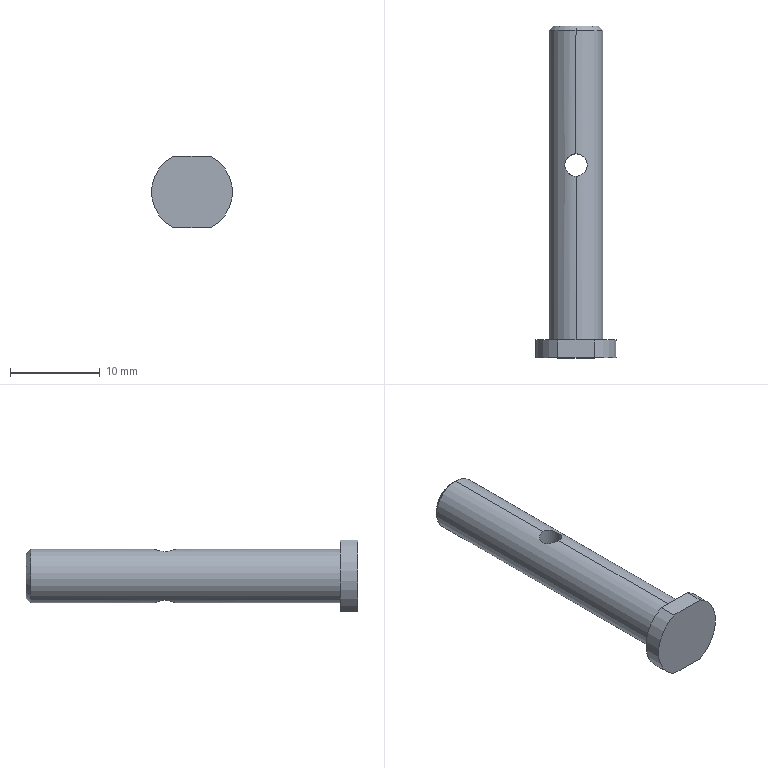Part | STEP file | 02-15 tensioning shaft | 1 solid | 13 faces | box 9 x 37 x 8 mm | volume 1080 mm3 | cylinder 6 | plane 5 | cone 2 | commonest cylinder face diameters 2.5 x2 6 x2 9 x2
STEP:
#1=CARTESIAN_POINT('',(0.,20.25,-3.));
#2=VERTEX_POINT('',#1);
#3=CARTESIAN_POINT('',(-1.25,21.5,-2.727));
#4=VERTEX_POINT('',#3);
#5=CARTESIAN_POINT('',(0.,20.25,-3.));
#6=CARTESIAN_POINT('',(-0.1646,20.25,-3.));
#7=CARTESIAN_POINT('',(-0.3304,20.283,-2.986));
#8=CARTESIAN_POINT('',(-0.6332,20.41,-2.936));
#9=CARTESIAN_POINT('',(-0.7698,20.502,-2.902));
#10=CARTESIAN_POINT('',(-0.9422,20.675,-2.849));
#11=CARTESIAN_POINT('',(-0.9933,20.737,-2.831));
#12=CARTESIAN_POINT('',(-1.083,20.871,-2.798));
#13=CARTESIAN_POINT('',(-1.122,20.944,-2.782));
#14=CARTESIAN_POINT('',(-1.185,21.094,-2.756));
#15=CARTESIAN_POINT('',(-1.209,21.172,-2.746));
#16=CARTESIAN_POINT('',(-1.242,21.334,-2.731));
#17=CARTESIAN_POINT('',(-1.25,21.418,-2.727));
#18=CARTESIAN_POINT('',(-1.25,21.5,-2.727));
#19=B_SPLINE_CURVE_WITH_KNOTS('',3,(#5,#6,#7,#8,#9,#10,#11,#12,#13,#14,#15,#16,#17,#18),.UNSPECIFIED.,.F.,.F.,(4,2,2,2,2,2,4),(0.003954,0.004448,0.004941,0.005188,0.005435,0.005682,0.005929),.UNSPECIFIED.);
#20=EDGE_CURVE('',#2,#4,#19,.T.);
#21=ORIENTED_EDGE('',*,*,#20,.T.);
#22=CARTESIAN_POINT('',(-1.25,21.5,2.727));
#23=VERTEX_POINT('',#22);
#24=CARTESIAN_POINT('',(-1.25,21.5,-6.));
#25=DIRECTION('',(0.,0.,1.));
#26=VECTOR('',#25,1000.);
#27=LINE('',#24,#26);
#28=EDGE_CURVE('',#4,#23,#27,.T.);
#29=ORIENTED_EDGE('',*,*,#28,.T.);
#30=CARTESIAN_POINT('',(0.,20.25,3.));
#31=VERTEX_POINT('',#30);
#32=CARTESIAN_POINT('',(-1.25,21.5,2.727));
#33=CARTESIAN_POINT('',(-1.25,21.335,2.727));
#34=CARTESIAN_POINT('',(-1.217,21.17,2.743));
#35=CARTESIAN_POINT('',(-1.09,20.867,2.796));
#36=CARTESIAN_POINT('',(-0.9986,20.731,2.831));
#37=CARTESIAN_POINT('',(-0.8261,20.558,2.885));
#38=CARTESIAN_POINT('',(-0.7638,20.507,2.902));
#39=CARTESIAN_POINT('',(-0.6296,20.417,2.934));
#40=CARTESIAN_POINT('',(-0.5566,20.378,2.949));
#41=CARTESIAN_POINT('',(-0.4058,20.315,2.973));
#42=CARTESIAN_POINT('',(-0.3277,20.291,2.983));
#43=CARTESIAN_POINT('',(-0.1662,20.258,2.996));
#44=CARTESIAN_POINT('',(-0.08241,20.25,3.));
#45=CARTESIAN_POINT('',(0.,20.25,3.));
#46=B_SPLINE_CURVE_WITH_KNOTS('',3,(#32,#33,#34,#35,#36,#37,#38,#39,#40,#41,#42,#43,#44,#45),.UNSPECIFIED.,.F.,.F.,(4,2,2,2,2,2,4),(0.003953,0.004447,0.004941,0.005188,0.005435,0.005682,0.005929),.UNSPECIFIED.);
#47=EDGE_CURVE('',#23,#31,#46,.T.);
#48=ORIENTED_EDGE('',*,*,#47,.T.);
#49=CARTESIAN_POINT('',(1.25,21.5,2.727));
#50=VERTEX_POINT('',#49);
#51=CARTESIAN_POINT('',(0.,20.25,3.));
#52=CARTESIAN_POINT('',(0.1648,20.25,3.));
#53=CARTESIAN_POINT('',(0.3309,20.284,2.986));
#54=CARTESIAN_POINT('',(0.6322,20.409,2.937));
#55=CARTESIAN_POINT('',(0.7695,20.502,2.902));
#56=CARTESIAN_POINT('',(0.9988,20.731,2.831));
#57=CARTESIAN_POINT('',(1.09,20.866,2.796));
#58=CARTESIAN_POINT('',(1.217,21.171,2.743));
#59=CARTESIAN_POINT('',(1.25,21.333,2.727));
#60=CARTESIAN_POINT('',(1.25,21.5,2.727));
#61=B_SPLINE_CURVE_WITH_KNOTS('',3,(#51,#52,#53,#54,#55,#56,#57,#58,#59,#60),.UNSPECIFIED.,.F.,.F.,(4,2,2,2,4),(0.005929,0.006423,0.006916,0.00741,0.007904),.UNSPECIFIED.);
#62=EDGE_CURVE('',#31,#50,#61,.T.);
#63=ORIENTED_EDGE('',*,*,#62,.T.);
#64=CARTESIAN_POINT('',(1.25,21.5,-2.727));
#65=VERTEX_POINT('',#64);
#66=CARTESIAN_POINT('',(1.25,21.5,-6.));
#67=DIRECTION('',(0.,0.,1.));
#68=VECTOR('',#67,1000.);
#69=LINE('',#66,#68);
#70=EDGE_CURVE('',#65,#50,#69,.T.);
#71=ORIENTED_EDGE('',*,*,#70,.F.);
#72=CARTESIAN_POINT('',(1.25,21.5,-2.727));
#73=CARTESIAN_POINT('',(1.25,21.417,-2.727));
#74=CARTESIAN_POINT('',(1.242,21.334,-2.731));
#75=CARTESIAN_POINT('',(1.209,21.172,-2.746));
#76=CARTESIAN_POINT('',(1.185,21.094,-2.756));
#77=CARTESIAN_POINT('',(1.09,20.866,-2.796));
#78=CARTESIAN_POINT('',(0.9976,20.73,-2.832));
#79=CARTESIAN_POINT('',(0.7691,20.501,-2.902));
#80=CARTESIAN_POINT('',(0.6313,20.409,-2.937));
#81=CARTESIAN_POINT('',(0.3309,20.284,-2.986));
#82=CARTESIAN_POINT('',(0.1647,20.25,-3.));
#83=CARTESIAN_POINT('',(0.,20.25,-3.));
#84=B_SPLINE_CURVE_WITH_KNOTS('',3,(#72,#73,#74,#75,#76,#77,#78,#79,#80,#81,#82,#83),.UNSPECIFIED.,.F.,.F.,(4,2,2,2,2,4),(0.001978,0.002225,0.002472,0.002966,0.00346,0.003954),.UNSPECIFIED.);
#85=EDGE_CURVE('',#65,#2,#84,.T.);
#86=ORIENTED_EDGE('',*,*,#85,.T.);
#87=EDGE_LOOP('',(#21,#29,#48,#63,#71,#86));
#88=FACE_OUTER_BOUND('',#87,.T.);
#89=CARTESIAN_POINT('',(0.,21.5,-6.));
#90=DIRECTION('',(0.,0.,1.));
#91=DIRECTION('',(1.,0.,0.));
#92=AXIS2_PLACEMENT_3D('',#89,#90,#91);
#93=CYLINDRICAL_SURFACE('',#92,1.25);
#94=ADVANCED_FACE('',(#88),#93,.F.);
#95=CARTESIAN_POINT('',(0.,37.,2.5));
#96=VERTEX_POINT('',#95);
#97=CARTESIAN_POINT('',(0.,37.,-2.5));
#98=VERTEX_POINT('',#97);
#99=CARTESIAN_POINT('',(0.,37.,0.));
#100=DIRECTION('',(0.,1.,0.));
#101=DIRECTION('',(0.,0.,1.));
#102=AXIS2_PLACEMENT_3D('',#99,#100,#101);
#103=CIRCLE('',#102,2.5);
#104=EDGE_CURVE('',#96,#98,#103,.T.);
#105=ORIENTED_EDGE('',*,*,#104,.F.);
#106=CARTESIAN_POINT('',(0.,36.5,3.));
#107=VERTEX_POINT('',#106);
#108=CARTESIAN_POINT('',(0.,36.5,3.));
#109=DIRECTION('',(0.,-0.7071,0.7071));
#110=VECTOR('',#109,1000.);
#111=LINE('',#108,#110);
#112=EDGE_CURVE('',#96,#107,#111,.T.);
#113=ORIENTED_EDGE('',*,*,#112,.T.);
#114=CARTESIAN_POINT('',(0.,36.5,-3.));
#115=VERTEX_POINT('',#114);
#116=CARTESIAN_POINT('',(0.,36.5,0.));
#117=DIRECTION('',(0.,-1.,0.));
#118=DIRECTION('',(0.,0.,1.));
#119=AXIS2_PLACEMENT_3D('',#116,#117,#118);
#120=CIRCLE('',#119,3.);
#121=EDGE_CURVE('',#115,#107,#120,.T.);
#122=ORIENTED_EDGE('',*,*,#121,.F.);
#123=CARTESIAN_POINT('',(0.,36.5,-3.));
#124=DIRECTION('',(0.,-0.7071,-0.7071));
#125=VECTOR('',#124,1000.);
#126=LINE('',#123,#125);
#127=EDGE_CURVE('',#98,#115,#126,.T.);
#128=ORIENTED_EDGE('',*,*,#127,.F.);
#129=EDGE_LOOP('',(#105,#113,#122,#128));
#130=FACE_OUTER_BOUND('',#129,.T.);
#131=CARTESIAN_POINT('',(0.,36.5,0.));
#132=DIRECTION('',(0.,-1.,0.));
#133=DIRECTION('',(0.,0.,-1.));
#134=AXIS2_PLACEMENT_3D('',#131,#132,#133);
#135=CONICAL_SURFACE('',#134,3.,0.7854);
#136=ADVANCED_FACE('',(#130),#135,.T.);
#137=ORIENTED_EDGE('',*,*,#121,.T.);
#138=CARTESIAN_POINT('',(0.,22.75,3.));
#139=VERTEX_POINT('',#138);
#140=CARTESIAN_POINT('',(0.,0.,3.));
#141=DIRECTION('',(0.,-1.,0.));
#142=VECTOR('',#141,1000.);
#143=LINE('',#140,#142);
#144=EDGE_CURVE('',#107,#139,#143,.T.);
#145=ORIENTED_EDGE('',*,*,#144,.T.);
#146=CARTESIAN_POINT('',(1.25,21.5,2.727));
#147=CARTESIAN_POINT('',(1.25,21.584,2.727));
#148=CARTESIAN_POINT('',(1.242,21.666,2.731));
#149=CARTESIAN_POINT('',(1.209,21.827,2.746));
#150=CARTESIAN_POINT('',(1.185,21.907,2.756));
#151=CARTESIAN_POINT('',(1.09,22.133,2.796));
#152=CARTESIAN_POINT('',(0.9976,22.27,2.832));
#153=CARTESIAN_POINT('',(0.7697,22.498,2.902));
#154=CARTESIAN_POINT('',(0.6318,22.591,2.937));
#155=CARTESIAN_POINT('',(0.3312,22.716,2.986));
#156=CARTESIAN_POINT('',(0.1654,22.75,3.));
#157=CARTESIAN_POINT('',(0.,22.75,3.));
#158=B_SPLINE_CURVE_WITH_KNOTS('',3,(#146,#147,#148,#149,#150,#151,#152,#153,#154,#155,#156,#157),.UNSPECIFIED.,.F.,.F.,(4,2,2,2,2,4),(0.,0.0002472,0.0004943,0.0009887,0.001483,0.001977),.UNSPECIFIED.);
#159=EDGE_CURVE('',#50,#139,#158,.T.);
#160=ORIENTED_EDGE('',*,*,#159,.F.);
#161=ORIENTED_EDGE('',*,*,#62,.F.);
#162=CARTESIAN_POINT('',(0.,2.,3.));
#163=VERTEX_POINT('',#162);
#164=CARTESIAN_POINT('',(0.,0.,3.));
#165=DIRECTION('',(0.,-1.,0.));
#166=VECTOR('',#165,1000.);
#167=LINE('',#164,#166);
#168=EDGE_CURVE('',#31,#163,#167,.T.);
#169=ORIENTED_EDGE('',*,*,#168,.T.);
#170=CARTESIAN_POINT('',(0.,2.,-3.));
#171=VERTEX_POINT('',#170);
#172=CARTESIAN_POINT('',(0.,2.,0.));
#173=DIRECTION('',(0.,-1.,0.));
#174=DIRECTION('',(0.,0.,-1.));
#175=AXIS2_PLACEMENT_3D('',#172,#173,#174);
#176=CIRCLE('',#175,3.);
#177=EDGE_CURVE('',#171,#163,#176,.T.);
#178=ORIENTED_EDGE('',*,*,#177,.F.);
#179=CARTESIAN_POINT('',(0.,0.,-3.));
#180=DIRECTION('',(0.,-1.,0.));
#181=VECTOR('',#180,1000.);
#182=LINE('',#179,#181);
#183=EDGE_CURVE('',#2,#171,#182,.T.);
#184=ORIENTED_EDGE('',*,*,#183,.F.);
#185=ORIENTED_EDGE('',*,*,#85,.F.);
#186=CARTESIAN_POINT('',(0.,22.75,-3.));
#187=VERTEX_POINT('',#186);
#188=CARTESIAN_POINT('',(0.,22.75,-3.));
#189=CARTESIAN_POINT('',(0.08365,22.75,-3.));
#190=CARTESIAN_POINT('',(0.1657,22.742,-2.997));
#191=CARTESIAN_POINT('',(0.3269,22.709,-2.983));
#192=CARTESIAN_POINT('',(0.4069,22.685,-2.973));
#193=CARTESIAN_POINT('',(0.6335,22.59,-2.936));
#194=CARTESIAN_POINT('',(0.7709,22.497,-2.902));
#195=CARTESIAN_POINT('',(0.9987,22.269,-2.831));
#196=CARTESIAN_POINT('',(1.091,22.131,-2.795));
#197=CARTESIAN_POINT('',(1.216,21.831,-2.743));
#198=CARTESIAN_POINT('',(1.25,21.665,-2.727));
#199=CARTESIAN_POINT('',(1.25,21.5,-2.727));
#200=B_SPLINE_CURVE_WITH_KNOTS('',3,(#188,#189,#190,#191,#192,#193,#194,#195,#196,#197,#198,#199),.UNSPECIFIED.,.F.,.F.,(4,2,2,2,2,4),(0.,0.0002472,0.0004944,0.0009888,0.001483,0.001978),.UNSPECIFIED.);
#201=EDGE_CURVE('',#187,#65,#200,.T.);
#202=ORIENTED_EDGE('',*,*,#201,.F.);
#203=CARTESIAN_POINT('',(0.,0.,-3.));
#204=DIRECTION('',(0.,-1.,0.));
#205=VECTOR('',#204,1000.);
#206=LINE('',#203,#205);
#207=EDGE_CURVE('',#115,#187,#206,.T.);
#208=ORIENTED_EDGE('',*,*,#207,.F.);
#209=EDGE_LOOP('',(#137,#145,#160,#161,#169,#178,#184,#185,#202,#208));
#210=FACE_OUTER_BOUND('',#209,.T.);
#211=CARTESIAN_POINT('',(0.,0.,0.));
#212=DIRECTION('',(0.,-1.,0.));
#213=DIRECTION('',(0.,0.,-1.));
#214=AXIS2_PLACEMENT_3D('',#211,#212,#213);
#215=CYLINDRICAL_SURFACE('',#214,3.);
#216=ADVANCED_FACE('',(#210),#215,.T.);
#217=CARTESIAN_POINT('',(2.062,0.,-4.));
#218=VERTEX_POINT('',#217);
#219=CARTESIAN_POINT('',(2.062,0.,4.));
#220=VERTEX_POINT('',#219);
#221=CARTESIAN_POINT('',(0.,0.,0.));
#222=DIRECTION('',(0.,-1.,0.));
#223=DIRECTION('',(0.,0.,-1.));
#224=AXIS2_PLACEMENT_3D('',#221,#222,#223);
#225=CIRCLE('',#224,4.5);
#226=EDGE_CURVE('',#218,#220,#225,.T.);
#227=ORIENTED_EDGE('',*,*,#226,.T.);
#228=CARTESIAN_POINT('',(-2.062,0.,4.));
#229=VERTEX_POINT('',#228);
#230=CARTESIAN_POINT('',(4.5,0.,4.));
#231=DIRECTION('',(-1.,0.,0.));
#232=VECTOR('',#231,1000.);
#233=LINE('',#230,#232);
#234=EDGE_CURVE('',#220,#229,#233,.T.);
#235=ORIENTED_EDGE('',*,*,#234,.T.);
#236=CARTESIAN_POINT('',(-2.062,0.,-4.));
#237=VERTEX_POINT('',#236);
#238=CARTESIAN_POINT('',(0.,0.,0.));
#239=DIRECTION('',(0.,-1.,0.));
#240=DIRECTION('',(0.,0.,-1.));
#241=AXIS2_PLACEMENT_3D('',#238,#239,#240);
#242=CIRCLE('',#241,4.5);
#243=EDGE_CURVE('',#229,#237,#242,.T.);
#244=ORIENTED_EDGE('',*,*,#243,.T.);
#245=CARTESIAN_POINT('',(4.5,0.,-4.));
#246=DIRECTION('',(1.,0.,0.));
#247=VECTOR('',#246,1000.);
#248=LINE('',#245,#247);
#249=EDGE_CURVE('',#237,#218,#248,.T.);
#250=ORIENTED_EDGE('',*,*,#249,.T.);
#251=EDGE_LOOP('',(#227,#235,#244,#250));
#252=FACE_OUTER_BOUND('',#251,.T.);
#253=CARTESIAN_POINT('',(0.,0.,0.));
#254=DIRECTION('',(0.,-1.,0.));
#255=DIRECTION('',(0.,0.,-1.));
#256=AXIS2_PLACEMENT_3D('',#253,#254,#255);
#257=PLANE('',#256);
#258=ADVANCED_FACE('',(#252),#257,.T.);
#259=CARTESIAN_POINT('',(-2.062,2.,4.));
#260=VERTEX_POINT('',#259);
#261=CARTESIAN_POINT('',(-2.062,2.,-4.));
#262=VERTEX_POINT('',#261);
#263=CARTESIAN_POINT('',(0.,2.,0.));
#264=DIRECTION('',(0.,-1.,0.));
#265=DIRECTION('',(0.,0.,-1.));
#266=AXIS2_PLACEMENT_3D('',#263,#264,#265);
#267=CIRCLE('',#266,4.5);
#268=EDGE_CURVE('',#260,#262,#267,.T.);
#269=ORIENTED_EDGE('',*,*,#268,.T.);
#270=CARTESIAN_POINT('',(-2.062,0.,-4.));
#271=DIRECTION('',(0.,-1.,0.));
#272=VECTOR('',#271,1000.);
#273=LINE('',#270,#272);
#274=EDGE_CURVE('',#262,#237,#273,.T.);
#275=ORIENTED_EDGE('',*,*,#274,.T.);
#276=ORIENTED_EDGE('',*,*,#243,.F.);
#277=CARTESIAN_POINT('',(-2.062,0.,4.));
#278=DIRECTION('',(0.,1.,0.));
#279=VECTOR('',#278,1000.);
#280=LINE('',#277,#279);
#281=EDGE_CURVE('',#229,#260,#280,.T.);
#282=ORIENTED_EDGE('',*,*,#281,.T.);
#283=EDGE_LOOP('',(#269,#275,#276,#282));
#284=FACE_OUTER_BOUND('',#283,.T.);
#285=CARTESIAN_POINT('',(0.,0.,0.));
#286=DIRECTION('',(0.,-1.,0.));
#287=DIRECTION('',(0.,0.,-1.));
#288=AXIS2_PLACEMENT_3D('',#285,#286,#287);
#289=CYLINDRICAL_SURFACE('',#288,4.5);
#290=ADVANCED_FACE('',(#284),#289,.T.);
#291=CARTESIAN_POINT('',(2.062,2.,-4.));
#292=VERTEX_POINT('',#291);
#293=CARTESIAN_POINT('',(2.062,2.,4.));
#294=VERTEX_POINT('',#293);
#295=CARTESIAN_POINT('',(0.,2.,0.));
#296=DIRECTION('',(0.,-1.,0.));
#297=DIRECTION('',(0.,0.,-1.));
#298=AXIS2_PLACEMENT_3D('',#295,#296,#297);
#299=CIRCLE('',#298,4.5);
#300=EDGE_CURVE('',#292,#294,#299,.T.);
#301=ORIENTED_EDGE('',*,*,#300,.T.);
#302=CARTESIAN_POINT('',(2.062,0.,4.));
#303=DIRECTION('',(0.,-1.,0.));
#304=VECTOR('',#303,1000.);
#305=LINE('',#302,#304);
#306=EDGE_CURVE('',#294,#220,#305,.T.);
#307=ORIENTED_EDGE('',*,*,#306,.T.);
#308=ORIENTED_EDGE('',*,*,#226,.F.);
#309=CARTESIAN_POINT('',(2.062,0.,-4.));
#310=DIRECTION('',(0.,1.,0.));
#311=VECTOR('',#310,1000.);
#312=LINE('',#309,#311);
#313=EDGE_CURVE('',#218,#292,#312,.T.);
#314=ORIENTED_EDGE('',*,*,#313,.T.);
#315=EDGE_LOOP('',(#301,#307,#308,#314));
#316=FACE_OUTER_BOUND('',#315,.T.);
#317=CARTESIAN_POINT('',(0.,0.,0.));
#318=DIRECTION('',(0.,-1.,0.));
#319=DIRECTION('',(0.,0.,-1.));
#320=AXIS2_PLACEMENT_3D('',#317,#318,#319);
#321=CYLINDRICAL_SURFACE('',#320,4.5);
#322=ADVANCED_FACE('',(#316),#321,.T.);
#323=ORIENTED_EDGE('',*,*,#177,.T.);
#324=CARTESIAN_POINT('',(0.,2.,0.));
#325=DIRECTION('',(0.,-1.,0.));
#326=DIRECTION('',(0.,0.,-1.));
#327=AXIS2_PLACEMENT_3D('',#324,#325,#326);
#328=CIRCLE('',#327,3.);
#329=EDGE_CURVE('',#163,#171,#328,.T.);
#330=ORIENTED_EDGE('',*,*,#329,.T.);
#331=EDGE_LOOP('',(#323,#330));
#332=FACE_BOUND('',#331,.T.);
#333=ORIENTED_EDGE('',*,*,#268,.F.);
#334=CARTESIAN_POINT('',(4.5,2.,4.));
#335=DIRECTION('',(1.,0.,0.));
#336=VECTOR('',#335,1000.);
#337=LINE('',#334,#336);
#338=EDGE_CURVE('',#260,#294,#337,.T.);
#339=ORIENTED_EDGE('',*,*,#338,.T.);
#340=ORIENTED_EDGE('',*,*,#300,.F.);
#341=CARTESIAN_POINT('',(4.5,2.,-4.));
#342=DIRECTION('',(-1.,0.,0.));
#343=VECTOR('',#342,1000.);
#344=LINE('',#341,#343);
#345=EDGE_CURVE('',#292,#262,#344,.T.);
#346=ORIENTED_EDGE('',*,*,#345,.T.);
#347=EDGE_LOOP('',(#333,#339,#340,#346));
#348=FACE_OUTER_BOUND('',#347,.T.);
#349=CARTESIAN_POINT('',(4.5,2.,0.));
#350=DIRECTION('',(0.,1.,0.));
#351=DIRECTION('',(0.,0.,1.));
#352=AXIS2_PLACEMENT_3D('',#349,#350,#351);
#353=PLANE('',#352);
#354=ADVANCED_FACE('',(#332,#348),#353,.T.);
#355=ORIENTED_EDGE('',*,*,#144,.F.);
#356=CARTESIAN_POINT('',(0.,36.5,0.));
#357=DIRECTION('',(0.,-1.,0.));
#358=DIRECTION('',(0.,0.,1.));
#359=AXIS2_PLACEMENT_3D('',#356,#357,#358);
#360=CIRCLE('',#359,3.);
#361=EDGE_CURVE('',#107,#115,#360,.T.);
#362=ORIENTED_EDGE('',*,*,#361,.T.);
#363=ORIENTED_EDGE('',*,*,#207,.T.);
#364=CARTESIAN_POINT('',(-1.25,21.5,-2.727));
#365=CARTESIAN_POINT('',(-1.25,21.665,-2.727));
#366=CARTESIAN_POINT('',(-1.216,21.831,-2.743));
#367=CARTESIAN_POINT('',(-1.091,22.132,-2.795));
#368=CARTESIAN_POINT('',(-0.999,22.269,-2.831));
#369=CARTESIAN_POINT('',(-0.7696,22.498,-2.902));
#370=CARTESIAN_POINT('',(-0.6343,22.59,-2.936));
#371=CARTESIAN_POINT('',(-0.3295,22.717,-2.986));
#372=CARTESIAN_POINT('',(-0.1671,22.75,-3.));
#373=CARTESIAN_POINT('',(0.,22.75,-3.));
#374=B_SPLINE_CURVE_WITH_KNOTS('',3,(#364,#365,#366,#367,#368,#369,#370,#371,#372,#373),.UNSPECIFIED.,.F.,.F.,(4,2,2,2,4),(0.005929,0.006423,0.006917,0.00741,0.007904),.UNSPECIFIED.);
#375=EDGE_CURVE('',#4,#187,#374,.T.);
#376=ORIENTED_EDGE('',*,*,#375,.F.);
#377=ORIENTED_EDGE('',*,*,#20,.F.);
#378=ORIENTED_EDGE('',*,*,#183,.T.);
#379=ORIENTED_EDGE('',*,*,#329,.F.);
#380=ORIENTED_EDGE('',*,*,#168,.F.);
#381=ORIENTED_EDGE('',*,*,#47,.F.);
#382=CARTESIAN_POINT('',(0.,22.75,3.));
#383=CARTESIAN_POINT('',(-0.08265,22.75,3.));
#384=CARTESIAN_POINT('',(-0.1664,22.742,2.996));
#385=CARTESIAN_POINT('',(-0.3276,22.709,2.983));
#386=CARTESIAN_POINT('',(-0.4063,22.685,2.973));
#387=CARTESIAN_POINT('',(-0.6347,22.589,2.936));
#388=CARTESIAN_POINT('',(-0.771,22.497,2.902));
#389=CARTESIAN_POINT('',(-0.9991,22.268,2.831));
#390=CARTESIAN_POINT('',(-1.091,22.131,2.795));
#391=CARTESIAN_POINT('',(-1.216,21.831,2.743));
#392=CARTESIAN_POINT('',(-1.25,21.665,2.727));
#393=CARTESIAN_POINT('',(-1.25,21.5,2.727));
#394=B_SPLINE_CURVE_WITH_KNOTS('',3,(#382,#383,#384,#385,#386,#387,#388,#389,#390,#391,#392,#393),.UNSPECIFIED.,.F.,.F.,(4,2,2,2,2,4),(0.001977,0.002224,0.002471,0.002965,0.003459,0.003953),.UNSPECIFIED.);
#395=EDGE_CURVE('',#139,#23,#394,.T.);
#396=ORIENTED_EDGE('',*,*,#395,.F.);
#397=EDGE_LOOP('',(#355,#362,#363,#376,#377,#378,#379,#380,#381,#396));
#398=FACE_OUTER_BOUND('',#397,.T.);
#399=CARTESIAN_POINT('',(0.,0.,0.));
#400=DIRECTION('',(0.,-1.,0.));
#401=DIRECTION('',(0.,0.,-1.));
#402=AXIS2_PLACEMENT_3D('',#399,#400,#401);
#403=CYLINDRICAL_SURFACE('',#402,3.);
#404=ADVANCED_FACE('',(#398),#403,.T.);
#405=CARTESIAN_POINT('',(0.,37.,0.));
#406=DIRECTION('',(0.,1.,0.));
#407=DIRECTION('',(0.,0.,1.));
#408=AXIS2_PLACEMENT_3D('',#405,#406,#407);
#409=CIRCLE('',#408,2.5);
#410=EDGE_CURVE('',#98,#96,#409,.T.);
#411=ORIENTED_EDGE('',*,*,#410,.T.);
#412=ORIENTED_EDGE('',*,*,#104,.T.);
#413=EDGE_LOOP('',(#411,#412));
#414=FACE_OUTER_BOUND('',#413,.T.);
#415=CARTESIAN_POINT('',(3.,37.,0.));
#416=DIRECTION('',(0.,1.,0.));
#417=DIRECTION('',(0.,0.,1.));
#418=AXIS2_PLACEMENT_3D('',#415,#416,#417);
#419=PLANE('',#418);
#420=ADVANCED_FACE('',(#414),#419,.T.);
#421=ORIENTED_EDGE('',*,*,#112,.F.);
#422=ORIENTED_EDGE('',*,*,#410,.F.);
#423=ORIENTED_EDGE('',*,*,#127,.T.);
#424=ORIENTED_EDGE('',*,*,#361,.F.);
#425=EDGE_LOOP('',(#421,#422,#423,#424));
#426=FACE_OUTER_BOUND('',#425,.T.);
#427=CARTESIAN_POINT('',(0.,36.5,0.));
#428=DIRECTION('',(0.,-1.,0.));
#429=DIRECTION('',(0.,0.,-1.));
#430=AXIS2_PLACEMENT_3D('',#427,#428,#429);
#431=CONICAL_SURFACE('',#430,3.,0.7854);
#432=ADVANCED_FACE('',(#426),#431,.T.);
#433=ORIENTED_EDGE('',*,*,#249,.F.);
#434=ORIENTED_EDGE('',*,*,#274,.F.);
#435=ORIENTED_EDGE('',*,*,#345,.F.);
#436=ORIENTED_EDGE('',*,*,#313,.F.);
#437=EDGE_LOOP('',(#433,#434,#435,#436));
#438=FACE_OUTER_BOUND('',#437,.T.);
#439=CARTESIAN_POINT('',(4.5,10.,-4.));
#440=DIRECTION('',(0.,0.,-1.));
#441=DIRECTION('',(-1.,0.,0.));
#442=AXIS2_PLACEMENT_3D('',#439,#440,#441);
#443=PLANE('',#442);
#444=ADVANCED_FACE('',(#438),#443,.T.);
#445=ORIENTED_EDGE('',*,*,#234,.F.);
#446=ORIENTED_EDGE('',*,*,#306,.F.);
#447=ORIENTED_EDGE('',*,*,#338,.F.);
#448=ORIENTED_EDGE('',*,*,#281,.F.);
#449=EDGE_LOOP('',(#445,#446,#447,#448));
#450=FACE_OUTER_BOUND('',#449,.T.);
#451=CARTESIAN_POINT('',(4.5,10.,4.));
#452=DIRECTION('',(0.,0.,1.));
#453=DIRECTION('',(1.,0.,0.));
#454=AXIS2_PLACEMENT_3D('',#451,#452,#453);
#455=PLANE('',#454);
#456=ADVANCED_FACE('',(#450),#455,.T.);
#457=ORIENTED_EDGE('',*,*,#28,.F.);
#458=ORIENTED_EDGE('',*,*,#375,.T.);
#459=ORIENTED_EDGE('',*,*,#201,.T.);
#460=ORIENTED_EDGE('',*,*,#70,.T.);
#461=ORIENTED_EDGE('',*,*,#159,.T.);
#462=ORIENTED_EDGE('',*,*,#395,.T.);
#463=EDGE_LOOP('',(#457,#458,#459,#460,#461,#462));
#464=FACE_OUTER_BOUND('',#463,.T.);
#465=CARTESIAN_POINT('',(0.,21.5,-6.));
#466=DIRECTION('',(0.,0.,1.));
#467=DIRECTION('',(1.,0.,0.));
#468=AXIS2_PLACEMENT_3D('',#465,#466,#467);
#469=CYLINDRICAL_SURFACE('',#468,1.25);
#470=ADVANCED_FACE('',(#464),#469,.F.);
#471=CLOSED_SHELL('',(#94,#136,#216,#258,#290,#322,#354,#404,#420,#432,#444,#456,#470));
#472=MANIFOLD_SOLID_BREP('',#471);
#473=CARTESIAN_POINT('',(0.,0.,0.));
#474=DIRECTION('',(0.,0.,1.));
#475=DIRECTION('',(1.,0.,0.));
#476=AXIS2_PLACEMENT_3D('',#473,#474,#475);
#477=(LENGTH_UNIT()NAMED_UNIT(*)SI_UNIT(.MILLI.,.METRE.));
#478=UNCERTAINTY_MEASURE_WITH_UNIT(LENGTH_MEASURE(0.00001),#477,'','');
#479=(NAMED_UNIT(*)PLANE_ANGLE_UNIT()SI_UNIT($,.RADIAN.));
#480=(NAMED_UNIT(*)SI_UNIT($,.STERADIAN.)SOLID_ANGLE_UNIT());
#481=(GEOMETRIC_REPRESENTATION_CONTEXT(3)GLOBAL_UNCERTAINTY_ASSIGNED_CONTEXT((#478))GLOBAL_UNIT_ASSIGNED_CONTEXT((#477,#479,#480))REPRESENTATION_CONTEXT('',''));
#482=ADVANCED_BREP_SHAPE_REPRESENTATION('',(#472,#476),#481);